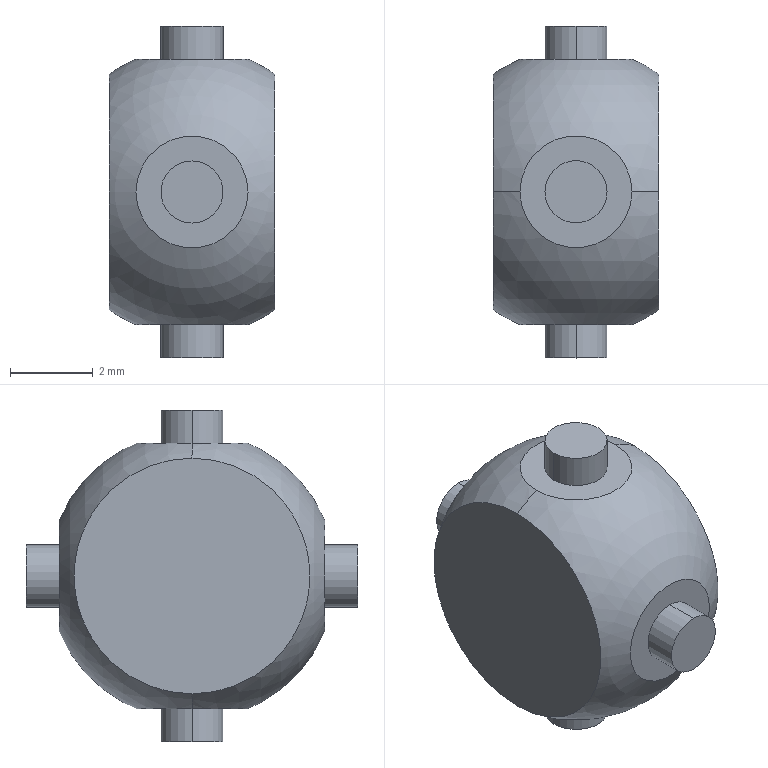Part | SolidWorks | features BaseBody 1, Scale 1 | 1 solid | 20 faces | box 4 x 8 x 8 mm | volume 137.312 mm3 | plane 10 | cylinder 8 | sphere 2 | commonest cylinder face diameters 1.5 x8
STEP:
#1=CARTESIAN_POINT('',(1.35,3.2,0.));
#2=VERTEX_POINT('',#1);
#3=CARTESIAN_POINT('',(-1.35,3.2,0.));
#4=VERTEX_POINT('',#3);
#5=CARTESIAN_POINT('',(0.,3.2,0.));
#6=DIRECTION('',(0.,1.,0.));
#7=DIRECTION('',(1.,0.,0.));
#8=AXIS2_PLACEMENT_3D('',#5,#6,#7);
#9=CIRCLE('',#8,1.35);
#10=EDGE_CURVE('',#2,#4,#9,.T.);
#11=ORIENTED_EDGE('',*,*,#10,.F.);
#12=CARTESIAN_POINT('',(0.,3.2,0.));
#13=DIRECTION('',(0.,1.,0.));
#14=DIRECTION('',(1.,0.,0.));
#15=AXIS2_PLACEMENT_3D('',#12,#13,#14);
#16=CIRCLE('',#15,1.35);
#17=EDGE_CURVE('',#4,#2,#16,.T.);
#18=ORIENTED_EDGE('',*,*,#17,.F.);
#19=EDGE_LOOP('',(#11,#18));
#20=FACE_BOUND('',#19,.T.);
#21=CARTESIAN_POINT('',(1.35,0.,-3.2));
#22=VERTEX_POINT('',#21);
#23=CARTESIAN_POINT('',(-1.35,0.,-3.2));
#24=VERTEX_POINT('',#23);
#25=CARTESIAN_POINT('',(0.,0.,-3.2));
#26=DIRECTION('',(0.,0.,1.));
#27=DIRECTION('',(1.,0.,0.));
#28=AXIS2_PLACEMENT_3D('',#25,#26,#27);
#29=CIRCLE('',#28,1.35);
#30=EDGE_CURVE('',#22,#24,#29,.T.);
#31=ORIENTED_EDGE('',*,*,#30,.T.);
#32=CARTESIAN_POINT('',(-2.,0.,-2.839));
#33=VERTEX_POINT('',#32);
#34=CARTESIAN_POINT('',(0.,0.,0.));
#35=DIRECTION('',(0.,1.,0.));
#36=DIRECTION('',(-1.,0.,0.));
#37=AXIS2_PLACEMENT_3D('',#34,#35,#36);
#38=CIRCLE('',#37,3.473);
#39=EDGE_CURVE('',#24,#33,#38,.T.);
#40=ORIENTED_EDGE('',*,*,#39,.T.);
#41=CARTESIAN_POINT('',(-2.,0.,2.839));
#42=VERTEX_POINT('',#41);
#43=CARTESIAN_POINT('',(-2.,0.,0.));
#44=DIRECTION('',(-1.,0.,0.));
#45=DIRECTION('',(0.,0.,-1.));
#46=AXIS2_PLACEMENT_3D('',#43,#44,#45);
#47=CIRCLE('',#46,2.839);
#48=EDGE_CURVE('',#42,#33,#47,.T.);
#49=ORIENTED_EDGE('',*,*,#48,.F.);
#50=CARTESIAN_POINT('',(-1.35,0.,3.2));
#51=VERTEX_POINT('',#50);
#52=CARTESIAN_POINT('',(0.,0.,0.));
#53=DIRECTION('',(0.,1.,0.));
#54=DIRECTION('',(-1.,0.,0.));
#55=AXIS2_PLACEMENT_3D('',#52,#53,#54);
#56=CIRCLE('',#55,3.473);
#57=EDGE_CURVE('',#42,#51,#56,.T.);
#58=ORIENTED_EDGE('',*,*,#57,.T.);
#59=CARTESIAN_POINT('',(1.35,0.,3.2));
#60=VERTEX_POINT('',#59);
#61=CARTESIAN_POINT('',(0.,0.,3.2));
#62=DIRECTION('',(0.,0.,1.));
#63=DIRECTION('',(1.,0.,0.));
#64=AXIS2_PLACEMENT_3D('',#61,#62,#63);
#65=CIRCLE('',#64,1.35);
#66=EDGE_CURVE('',#60,#51,#65,.T.);
#67=ORIENTED_EDGE('',*,*,#66,.F.);
#68=CARTESIAN_POINT('',(2.,0.,2.839));
#69=VERTEX_POINT('',#68);
#70=CARTESIAN_POINT('',(0.,0.,0.));
#71=DIRECTION('',(0.,-1.,0.));
#72=DIRECTION('',(0.,0.,-1.));
#73=AXIS2_PLACEMENT_3D('',#70,#71,#72);
#74=CIRCLE('',#73,3.473);
#75=EDGE_CURVE('',#69,#60,#74,.T.);
#76=ORIENTED_EDGE('',*,*,#75,.F.);
#77=CARTESIAN_POINT('',(2.,0.,-2.839));
#78=VERTEX_POINT('',#77);
#79=CARTESIAN_POINT('',(2.,0.,0.));
#80=DIRECTION('',(1.,0.,0.));
#81=DIRECTION('',(0.,0.,1.));
#82=AXIS2_PLACEMENT_3D('',#79,#80,#81);
#83=CIRCLE('',#82,2.839);
#84=EDGE_CURVE('',#78,#69,#83,.T.);
#85=ORIENTED_EDGE('',*,*,#84,.F.);
#86=CARTESIAN_POINT('',(0.,0.,0.));
#87=DIRECTION('',(0.,-1.,0.));
#88=DIRECTION('',(0.,0.,-1.));
#89=AXIS2_PLACEMENT_3D('',#86,#87,#88);
#90=CIRCLE('',#89,3.473);
#91=EDGE_CURVE('',#22,#78,#90,.T.);
#92=ORIENTED_EDGE('',*,*,#91,.F.);
#93=EDGE_LOOP('',(#31,#40,#49,#58,#67,#76,#85,#92));
#94=FACE_OUTER_BOUND('',#93,.T.);
#95=CARTESIAN_POINT('',(0.,0.,0.));
#96=DIRECTION('',(0.,1.,0.));
#97=DIRECTION('',(1.,0.,0.));
#98=AXIS2_PLACEMENT_3D('',#95,#96,#97);
#99=SPHERICAL_SURFACE('',#98,3.473);
#100=ADVANCED_FACE('',(#20,#94),#99,.T.);
#101=CARTESIAN_POINT('',(0.,3.2,-0.75));
#102=VERTEX_POINT('',#101);
#103=CARTESIAN_POINT('',(0.,3.2,0.75));
#104=VERTEX_POINT('',#103);
#105=CARTESIAN_POINT('',(0.,3.2,0.));
#106=DIRECTION('',(0.,-1.,0.));
#107=DIRECTION('',(1.,0.,0.));
#108=AXIS2_PLACEMENT_3D('',#105,#106,#107);
#109=CIRCLE('',#108,0.75);
#110=EDGE_CURVE('',#102,#104,#109,.T.);
#111=ORIENTED_EDGE('',*,*,#110,.F.);
#112=CARTESIAN_POINT('',(0.,4.,-0.75));
#113=VERTEX_POINT('',#112);
#114=CARTESIAN_POINT('',(0.,-4.,-0.75));
#115=DIRECTION('',(0.,1.,0.));
#116=VECTOR('',#115,1000.);
#117=LINE('',#114,#116);
#118=EDGE_CURVE('',#102,#113,#117,.T.);
#119=ORIENTED_EDGE('',*,*,#118,.T.);
#120=CARTESIAN_POINT('',(0.,4.,0.75));
#121=VERTEX_POINT('',#120);
#122=CARTESIAN_POINT('',(0.,4.,0.));
#123=DIRECTION('',(0.,1.,0.));
#124=DIRECTION('',(1.,0.,0.));
#125=AXIS2_PLACEMENT_3D('',#122,#123,#124);
#126=CIRCLE('',#125,0.75);
#127=EDGE_CURVE('',#121,#113,#126,.T.);
#128=ORIENTED_EDGE('',*,*,#127,.F.);
#129=CARTESIAN_POINT('',(0.,-4.,0.75));
#130=DIRECTION('',(0.,1.,0.));
#131=VECTOR('',#130,1000.);
#132=LINE('',#129,#131);
#133=EDGE_CURVE('',#104,#121,#132,.T.);
#134=ORIENTED_EDGE('',*,*,#133,.F.);
#135=EDGE_LOOP('',(#111,#119,#128,#134));
#136=FACE_OUTER_BOUND('',#135,.T.);
#137=CARTESIAN_POINT('',(0.,-4.,0.));
#138=DIRECTION('',(0.,1.,0.));
#139=DIRECTION('',(0.,0.,1.));
#140=AXIS2_PLACEMENT_3D('',#137,#138,#139);
#141=CYLINDRICAL_SURFACE('',#140,0.75);
#142=ADVANCED_FACE('',(#136),#141,.T.);
#143=CARTESIAN_POINT('',(0.,-4.,0.75));
#144=VERTEX_POINT('',#143);
#145=CARTESIAN_POINT('',(0.,-4.,-0.75));
#146=VERTEX_POINT('',#145);
#147=CARTESIAN_POINT('',(0.,-4.,0.));
#148=DIRECTION('',(0.,1.,0.));
#149=DIRECTION('',(1.,0.,0.));
#150=AXIS2_PLACEMENT_3D('',#147,#148,#149);
#151=CIRCLE('',#150,0.75);
#152=EDGE_CURVE('',#144,#146,#151,.T.);
#153=ORIENTED_EDGE('',*,*,#152,.T.);
#154=CARTESIAN_POINT('',(0.,-3.2,-0.75));
#155=VERTEX_POINT('',#154);
#156=CARTESIAN_POINT('',(0.,-4.,-0.75));
#157=DIRECTION('',(0.,1.,0.));
#158=VECTOR('',#157,1000.);
#159=LINE('',#156,#158);
#160=EDGE_CURVE('',#146,#155,#159,.T.);
#161=ORIENTED_EDGE('',*,*,#160,.T.);
#162=CARTESIAN_POINT('',(0.,-3.2,0.75));
#163=VERTEX_POINT('',#162);
#164=CARTESIAN_POINT('',(0.,-3.2,0.));
#165=DIRECTION('',(0.,1.,0.));
#166=DIRECTION('',(-1.,0.,0.));
#167=AXIS2_PLACEMENT_3D('',#164,#165,#166);
#168=CIRCLE('',#167,0.75);
#169=EDGE_CURVE('',#163,#155,#168,.T.);
#170=ORIENTED_EDGE('',*,*,#169,.F.);
#171=CARTESIAN_POINT('',(0.,-4.,0.75));
#172=DIRECTION('',(0.,1.,0.));
#173=VECTOR('',#172,1000.);
#174=LINE('',#171,#173);
#175=EDGE_CURVE('',#144,#163,#174,.T.);
#176=ORIENTED_EDGE('',*,*,#175,.F.);
#177=EDGE_LOOP('',(#153,#161,#170,#176));
#178=FACE_OUTER_BOUND('',#177,.T.);
#179=CARTESIAN_POINT('',(0.,-4.,0.));
#180=DIRECTION('',(0.,1.,0.));
#181=DIRECTION('',(0.,0.,1.));
#182=AXIS2_PLACEMENT_3D('',#179,#180,#181);
#183=CYLINDRICAL_SURFACE('',#182,0.75);
#184=ADVANCED_FACE('',(#178),#183,.T.);
#185=CARTESIAN_POINT('',(-0.75,0.,-3.2));
#186=VERTEX_POINT('',#185);
#187=CARTESIAN_POINT('',(0.75,0.,-3.2));
#188=VERTEX_POINT('',#187);
#189=CARTESIAN_POINT('',(0.,0.,-3.2));
#190=DIRECTION('',(0.,0.,-1.));
#191=DIRECTION('',(-1.,0.,0.));
#192=AXIS2_PLACEMENT_3D('',#189,#190,#191);
#193=CIRCLE('',#192,0.75);
#194=EDGE_CURVE('',#186,#188,#193,.T.);
#195=ORIENTED_EDGE('',*,*,#194,.T.);
#196=CARTESIAN_POINT('',(0.75,0.,-4.));
#197=VERTEX_POINT('',#196);
#198=CARTESIAN_POINT('',(0.75,0.,4.));
#199=DIRECTION('',(0.,0.,-1.));
#200=VECTOR('',#199,1000.);
#201=LINE('',#198,#200);
#202=EDGE_CURVE('',#188,#197,#201,.T.);
#203=ORIENTED_EDGE('',*,*,#202,.T.);
#204=CARTESIAN_POINT('',(-0.75,0.,-4.));
#205=VERTEX_POINT('',#204);
#206=CARTESIAN_POINT('',(0.,0.,-4.));
#207=DIRECTION('',(0.,0.,-1.));
#208=DIRECTION('',(1.,0.,0.));
#209=AXIS2_PLACEMENT_3D('',#206,#207,#208);
#210=CIRCLE('',#209,0.75);
#211=EDGE_CURVE('',#205,#197,#210,.T.);
#212=ORIENTED_EDGE('',*,*,#211,.F.);
#213=CARTESIAN_POINT('',(-0.75,0.,4.));
#214=DIRECTION('',(0.,0.,-1.));
#215=VECTOR('',#214,1000.);
#216=LINE('',#213,#215);
#217=EDGE_CURVE('',#186,#205,#216,.T.);
#218=ORIENTED_EDGE('',*,*,#217,.F.);
#219=EDGE_LOOP('',(#195,#203,#212,#218));
#220=FACE_OUTER_BOUND('',#219,.T.);
#221=CARTESIAN_POINT('',(0.,0.,4.));
#222=DIRECTION('',(0.,0.,-1.));
#223=DIRECTION('',(-1.,0.,0.));
#224=AXIS2_PLACEMENT_3D('',#221,#222,#223);
#225=CYLINDRICAL_SURFACE('',#224,0.75);
#226=ADVANCED_FACE('',(#220),#225,.T.);
#227=CARTESIAN_POINT('',(-0.75,0.,4.));
#228=VERTEX_POINT('',#227);
#229=CARTESIAN_POINT('',(0.75,0.,4.));
#230=VERTEX_POINT('',#229);
#231=CARTESIAN_POINT('',(0.,0.,4.));
#232=DIRECTION('',(0.,0.,-1.));
#233=DIRECTION('',(1.,0.,0.));
#234=AXIS2_PLACEMENT_3D('',#231,#232,#233);
#235=CIRCLE('',#234,0.75);
#236=EDGE_CURVE('',#228,#230,#235,.T.);
#237=ORIENTED_EDGE('',*,*,#236,.T.);
#238=CARTESIAN_POINT('',(0.75,0.,3.2));
#239=VERTEX_POINT('',#238);
#240=CARTESIAN_POINT('',(0.75,0.,4.));
#241=DIRECTION('',(0.,0.,-1.));
#242=VECTOR('',#241,1000.);
#243=LINE('',#240,#242);
#244=EDGE_CURVE('',#230,#239,#243,.T.);
#245=ORIENTED_EDGE('',*,*,#244,.T.);
#246=CARTESIAN_POINT('',(-0.75,0.,3.2));
#247=VERTEX_POINT('',#246);
#248=CARTESIAN_POINT('',(0.,0.,3.2));
#249=DIRECTION('',(0.,0.,1.));
#250=DIRECTION('',(1.,0.,0.));
#251=AXIS2_PLACEMENT_3D('',#248,#249,#250);
#252=CIRCLE('',#251,0.75);
#253=EDGE_CURVE('',#239,#247,#252,.T.);
#254=ORIENTED_EDGE('',*,*,#253,.T.);
#255=CARTESIAN_POINT('',(-0.75,0.,4.));
#256=DIRECTION('',(0.,0.,-1.));
#257=VECTOR('',#256,1000.);
#258=LINE('',#255,#257);
#259=EDGE_CURVE('',#228,#247,#258,.T.);
#260=ORIENTED_EDGE('',*,*,#259,.F.);
#261=EDGE_LOOP('',(#237,#245,#254,#260));
#262=FACE_OUTER_BOUND('',#261,.T.);
#263=CARTESIAN_POINT('',(0.,0.,4.));
#264=DIRECTION('',(0.,0.,-1.));
#265=DIRECTION('',(-1.,0.,0.));
#266=AXIS2_PLACEMENT_3D('',#263,#264,#265);
#267=CYLINDRICAL_SURFACE('',#266,0.75);
#268=ADVANCED_FACE('',(#262),#267,.T.);
#269=ORIENTED_EDGE('',*,*,#236,.F.);
#270=CARTESIAN_POINT('',(0.,0.,4.));
#271=DIRECTION('',(0.,0.,-1.));
#272=DIRECTION('',(1.,0.,0.));
#273=AXIS2_PLACEMENT_3D('',#270,#271,#272);
#274=CIRCLE('',#273,0.75);
#275=EDGE_CURVE('',#230,#228,#274,.T.);
#276=ORIENTED_EDGE('',*,*,#275,.F.);
#277=EDGE_LOOP('',(#269,#276));
#278=FACE_OUTER_BOUND('',#277,.T.);
#279=CARTESIAN_POINT('',(0.,0.,4.));
#280=DIRECTION('',(0.,0.,-1.));
#281=DIRECTION('',(0.,-1.,0.));
#282=AXIS2_PLACEMENT_3D('',#279,#280,#281);
#283=PLANE('',#282);
#284=ADVANCED_FACE('',(#278),#283,.F.);
#285=ORIENTED_EDGE('',*,*,#244,.F.);
#286=ORIENTED_EDGE('',*,*,#275,.T.);
#287=ORIENTED_EDGE('',*,*,#259,.T.);
#288=CARTESIAN_POINT('',(0.,0.,3.2));
#289=DIRECTION('',(0.,0.,1.));
#290=DIRECTION('',(1.,0.,0.));
#291=AXIS2_PLACEMENT_3D('',#288,#289,#290);
#292=CIRCLE('',#291,0.75);
#293=EDGE_CURVE('',#247,#239,#292,.T.);
#294=ORIENTED_EDGE('',*,*,#293,.T.);
#295=EDGE_LOOP('',(#285,#286,#287,#294));
#296=FACE_OUTER_BOUND('',#295,.T.);
#297=CARTESIAN_POINT('',(0.,0.,4.));
#298=DIRECTION('',(0.,0.,-1.));
#299=DIRECTION('',(-1.,0.,0.));
#300=AXIS2_PLACEMENT_3D('',#297,#298,#299);
#301=CYLINDRICAL_SURFACE('',#300,0.75);
#302=ADVANCED_FACE('',(#296),#301,.T.);
#303=ORIENTED_EDGE('',*,*,#202,.F.);
#304=CARTESIAN_POINT('',(0.,0.,-3.2));
#305=DIRECTION('',(0.,0.,-1.));
#306=DIRECTION('',(-1.,0.,0.));
#307=AXIS2_PLACEMENT_3D('',#304,#305,#306);
#308=CIRCLE('',#307,0.75);
#309=EDGE_CURVE('',#188,#186,#308,.T.);
#310=ORIENTED_EDGE('',*,*,#309,.T.);
#311=ORIENTED_EDGE('',*,*,#217,.T.);
#312=CARTESIAN_POINT('',(0.,0.,-4.));
#313=DIRECTION('',(0.,0.,-1.));
#314=DIRECTION('',(1.,0.,0.));
#315=AXIS2_PLACEMENT_3D('',#312,#313,#314);
#316=CIRCLE('',#315,0.75);
#317=EDGE_CURVE('',#197,#205,#316,.T.);
#318=ORIENTED_EDGE('',*,*,#317,.F.);
#319=EDGE_LOOP('',(#303,#310,#311,#318));
#320=FACE_OUTER_BOUND('',#319,.T.);
#321=CARTESIAN_POINT('',(0.,0.,4.));
#322=DIRECTION('',(0.,0.,-1.));
#323=DIRECTION('',(-1.,0.,0.));
#324=AXIS2_PLACEMENT_3D('',#321,#322,#323);
#325=CYLINDRICAL_SURFACE('',#324,0.75);
#326=ADVANCED_FACE('',(#320),#325,.T.);
#327=ORIENTED_EDGE('',*,*,#211,.T.);
#328=ORIENTED_EDGE('',*,*,#317,.T.);
#329=EDGE_LOOP('',(#327,#328));
#330=FACE_OUTER_BOUND('',#329,.T.);
#331=CARTESIAN_POINT('',(0.,0.,-4.));
#332=DIRECTION('',(0.,0.,-1.));
#333=DIRECTION('',(0.,-1.,0.));
#334=AXIS2_PLACEMENT_3D('',#331,#332,#333);
#335=PLANE('',#334);
#336=ADVANCED_FACE('',(#330),#335,.T.);
#337=ORIENTED_EDGE('',*,*,#152,.F.);
#338=CARTESIAN_POINT('',(0.,-4.,0.));
#339=DIRECTION('',(0.,1.,0.));
#340=DIRECTION('',(1.,0.,0.));
#341=AXIS2_PLACEMENT_3D('',#338,#339,#340);
#342=CIRCLE('',#341,0.75);
#343=EDGE_CURVE('',#146,#144,#342,.T.);
#344=ORIENTED_EDGE('',*,*,#343,.F.);
#345=EDGE_LOOP('',(#337,#344));
#346=FACE_OUTER_BOUND('',#345,.T.);
#347=CARTESIAN_POINT('',(0.,-4.,0.));
#348=DIRECTION('',(0.,1.,0.));
#349=DIRECTION('',(1.,0.,0.));
#350=AXIS2_PLACEMENT_3D('',#347,#348,#349);
#351=PLANE('',#350);
#352=ADVANCED_FACE('',(#346),#351,.F.);
#353=ORIENTED_EDGE('',*,*,#160,.F.);
#354=ORIENTED_EDGE('',*,*,#343,.T.);
#355=ORIENTED_EDGE('',*,*,#175,.T.);
#356=CARTESIAN_POINT('',(0.,-3.2,0.));
#357=DIRECTION('',(0.,1.,0.));
#358=DIRECTION('',(-1.,0.,0.));
#359=AXIS2_PLACEMENT_3D('',#356,#357,#358);
#360=CIRCLE('',#359,0.75);
#361=EDGE_CURVE('',#155,#163,#360,.T.);
#362=ORIENTED_EDGE('',*,*,#361,.F.);
#363=EDGE_LOOP('',(#353,#354,#355,#362));
#364=FACE_OUTER_BOUND('',#363,.T.);
#365=CARTESIAN_POINT('',(0.,-4.,0.));
#366=DIRECTION('',(0.,1.,0.));
#367=DIRECTION('',(0.,0.,1.));
#368=AXIS2_PLACEMENT_3D('',#365,#366,#367);
#369=CYLINDRICAL_SURFACE('',#368,0.75);
#370=ADVANCED_FACE('',(#364),#369,.T.);
#371=ORIENTED_EDGE('',*,*,#118,.F.);
#372=CARTESIAN_POINT('',(0.,3.2,0.));
#373=DIRECTION('',(0.,-1.,0.));
#374=DIRECTION('',(1.,0.,0.));
#375=AXIS2_PLACEMENT_3D('',#372,#373,#374);
#376=CIRCLE('',#375,0.75);
#377=EDGE_CURVE('',#104,#102,#376,.T.);
#378=ORIENTED_EDGE('',*,*,#377,.F.);
#379=ORIENTED_EDGE('',*,*,#133,.T.);
#380=CARTESIAN_POINT('',(0.,4.,0.));
#381=DIRECTION('',(0.,1.,0.));
#382=DIRECTION('',(1.,0.,0.));
#383=AXIS2_PLACEMENT_3D('',#380,#381,#382);
#384=CIRCLE('',#383,0.75);
#385=EDGE_CURVE('',#113,#121,#384,.T.);
#386=ORIENTED_EDGE('',*,*,#385,.F.);
#387=EDGE_LOOP('',(#371,#378,#379,#386));
#388=FACE_OUTER_BOUND('',#387,.T.);
#389=CARTESIAN_POINT('',(0.,-4.,0.));
#390=DIRECTION('',(0.,1.,0.));
#391=DIRECTION('',(0.,0.,1.));
#392=AXIS2_PLACEMENT_3D('',#389,#390,#391);
#393=CYLINDRICAL_SURFACE('',#392,0.75);
#394=ADVANCED_FACE('',(#388),#393,.T.);
#395=ORIENTED_EDGE('',*,*,#127,.T.);
#396=ORIENTED_EDGE('',*,*,#385,.T.);
#397=EDGE_LOOP('',(#395,#396));
#398=FACE_OUTER_BOUND('',#397,.T.);
#399=CARTESIAN_POINT('',(0.,4.,0.));
#400=DIRECTION('',(0.,1.,0.));
#401=DIRECTION('',(1.,0.,0.));
#402=AXIS2_PLACEMENT_3D('',#399,#400,#401);
#403=PLANE('',#402);
#404=ADVANCED_FACE('',(#398),#403,.T.);
#405=ORIENTED_EDGE('',*,*,#10,.T.);
#406=ORIENTED_EDGE('',*,*,#17,.T.);
#407=EDGE_LOOP('',(#405,#406));
#408=FACE_OUTER_BOUND('',#407,.T.);
#409=ORIENTED_EDGE('',*,*,#377,.T.);
#410=ORIENTED_EDGE('',*,*,#110,.T.);
#411=EDGE_LOOP('',(#409,#410));
#412=FACE_BOUND('',#411,.T.);
#413=CARTESIAN_POINT('',(2.,3.2,3.2));
#414=DIRECTION('',(0.,-1.,0.));
#415=DIRECTION('',(-1.,0.,0.));
#416=AXIS2_PLACEMENT_3D('',#413,#414,#415);
#417=PLANE('',#416);
#418=ADVANCED_FACE('',(#408,#412),#417,.F.);
#419=CARTESIAN_POINT('',(2.,0.,0.));
#420=DIRECTION('',(1.,0.,0.));
#421=DIRECTION('',(0.,0.,1.));
#422=AXIS2_PLACEMENT_3D('',#419,#420,#421);
#423=CIRCLE('',#422,2.839);
#424=EDGE_CURVE('',#69,#78,#423,.T.);
#425=ORIENTED_EDGE('',*,*,#424,.T.);
#426=ORIENTED_EDGE('',*,*,#84,.T.);
#427=EDGE_LOOP('',(#425,#426));
#428=FACE_OUTER_BOUND('',#427,.T.);
#429=CARTESIAN_POINT('',(2.,-3.2,3.2));
#430=DIRECTION('',(-1.,0.,0.));
#431=DIRECTION('',(0.,0.,1.));
#432=AXIS2_PLACEMENT_3D('',#429,#430,#431);
#433=PLANE('',#432);
#434=ADVANCED_FACE('',(#428),#433,.F.);
#435=CARTESIAN_POINT('',(-1.35,-3.2,0.));
#436=VERTEX_POINT('',#435);
#437=CARTESIAN_POINT('',(1.35,-3.2,0.));
#438=VERTEX_POINT('',#437);
#439=CARTESIAN_POINT('',(0.,-3.2,0.));
#440=DIRECTION('',(0.,-1.,0.));
#441=DIRECTION('',(-1.,0.,0.));
#442=AXIS2_PLACEMENT_3D('',#439,#440,#441);
#443=CIRCLE('',#442,1.35);
#444=EDGE_CURVE('',#436,#438,#443,.T.);
#445=ORIENTED_EDGE('',*,*,#444,.T.);
#446=CARTESIAN_POINT('',(0.,-3.2,0.));
#447=DIRECTION('',(0.,-1.,0.));
#448=DIRECTION('',(-1.,0.,0.));
#449=AXIS2_PLACEMENT_3D('',#446,#447,#448);
#450=CIRCLE('',#449,1.35);
#451=EDGE_CURVE('',#438,#436,#450,.T.);
#452=ORIENTED_EDGE('',*,*,#451,.T.);
#453=EDGE_LOOP('',(#445,#452));
#454=FACE_OUTER_BOUND('',#453,.T.);
#455=ORIENTED_EDGE('',*,*,#169,.T.);
#456=ORIENTED_EDGE('',*,*,#361,.T.);
#457=EDGE_LOOP('',(#455,#456));
#458=FACE_BOUND('',#457,.T.);
#459=CARTESIAN_POINT('',(-2.,-3.2,3.2));
#460=DIRECTION('',(0.,1.,0.));
#461=DIRECTION('',(1.,0.,0.));
#462=AXIS2_PLACEMENT_3D('',#459,#460,#461);
#463=PLANE('',#462);
#464=ADVANCED_FACE('',(#454,#458),#463,.F.);
#465=CARTESIAN_POINT('',(-2.,0.,0.));
#466=DIRECTION('',(-1.,0.,0.));
#467=DIRECTION('',(0.,0.,-1.));
#468=AXIS2_PLACEMENT_3D('',#465,#466,#467);
#469=CIRCLE('',#468,2.839);
#470=EDGE_CURVE('',#33,#42,#469,.T.);
#471=ORIENTED_EDGE('',*,*,#470,.T.);
#472=ORIENTED_EDGE('',*,*,#48,.T.);
#473=EDGE_LOOP('',(#471,#472));
#474=FACE_OUTER_BOUND('',#473,.T.);
#475=CARTESIAN_POINT('',(-2.,3.2,3.2));
#476=DIRECTION('',(1.,0.,0.));
#477=DIRECTION('',(0.,1.,0.));
#478=AXIS2_PLACEMENT_3D('',#475,#476,#477);
#479=PLANE('',#478);
#480=ADVANCED_FACE('',(#474),#479,.F.);
#481=ORIENTED_EDGE('',*,*,#30,.F.);
#482=CARTESIAN_POINT('',(0.,0.,-3.2));
#483=DIRECTION('',(0.,0.,1.));
#484=DIRECTION('',(1.,0.,0.));
#485=AXIS2_PLACEMENT_3D('',#482,#483,#484);
#486=CIRCLE('',#485,1.35);
#487=EDGE_CURVE('',#24,#22,#486,.T.);
#488=ORIENTED_EDGE('',*,*,#487,.F.);
#489=EDGE_LOOP('',(#481,#488));
#490=FACE_OUTER_BOUND('',#489,.T.);
#491=ORIENTED_EDGE('',*,*,#194,.F.);
#492=ORIENTED_EDGE('',*,*,#309,.F.);
#493=EDGE_LOOP('',(#491,#492));
#494=FACE_BOUND('',#493,.T.);
#495=CARTESIAN_POINT('',(0.,0.,-3.2));
#496=DIRECTION('',(0.,0.,-1.));
#497=DIRECTION('',(0.,-1.,0.));
#498=AXIS2_PLACEMENT_3D('',#495,#496,#497);
#499=PLANE('',#498);
#500=ADVANCED_FACE('',(#490,#494),#499,.T.);
#501=ORIENTED_EDGE('',*,*,#39,.F.);
#502=ORIENTED_EDGE('',*,*,#487,.T.);
#503=ORIENTED_EDGE('',*,*,#91,.T.);
#504=ORIENTED_EDGE('',*,*,#424,.F.);
#505=ORIENTED_EDGE('',*,*,#75,.T.);
#506=CARTESIAN_POINT('',(0.,0.,3.2));
#507=DIRECTION('',(0.,0.,1.));
#508=DIRECTION('',(1.,0.,0.));
#509=AXIS2_PLACEMENT_3D('',#506,#507,#508);
#510=CIRCLE('',#509,1.35);
#511=EDGE_CURVE('',#51,#60,#510,.T.);
#512=ORIENTED_EDGE('',*,*,#511,.F.);
#513=ORIENTED_EDGE('',*,*,#57,.F.);
#514=ORIENTED_EDGE('',*,*,#470,.F.);
#515=EDGE_LOOP('',(#501,#502,#503,#504,#505,#512,#513,#514));
#516=FACE_OUTER_BOUND('',#515,.T.);
#517=ORIENTED_EDGE('',*,*,#444,.F.);
#518=ORIENTED_EDGE('',*,*,#451,.F.);
#519=EDGE_LOOP('',(#517,#518));
#520=FACE_BOUND('',#519,.T.);
#521=CARTESIAN_POINT('',(0.,0.,0.));
#522=DIRECTION('',(0.,1.,0.));
#523=DIRECTION('',(1.,0.,0.));
#524=AXIS2_PLACEMENT_3D('',#521,#522,#523);
#525=SPHERICAL_SURFACE('',#524,3.473);
#526=ADVANCED_FACE('',(#516,#520),#525,.T.);
#527=ORIENTED_EDGE('',*,*,#66,.T.);
#528=ORIENTED_EDGE('',*,*,#511,.T.);
#529=EDGE_LOOP('',(#527,#528));
#530=FACE_OUTER_BOUND('',#529,.T.);
#531=ORIENTED_EDGE('',*,*,#293,.F.);
#532=ORIENTED_EDGE('',*,*,#253,.F.);
#533=EDGE_LOOP('',(#531,#532));
#534=FACE_BOUND('',#533,.T.);
#535=CARTESIAN_POINT('',(0.,0.,3.2));
#536=DIRECTION('',(0.,0.,1.));
#537=DIRECTION('',(1.,0.,0.));
#538=AXIS2_PLACEMENT_3D('',#535,#536,#537);
#539=PLANE('',#538);
#540=ADVANCED_FACE('',(#530,#534),#539,.T.);
#541=CLOSED_SHELL('',(#100,#142,#184,#226,#268,#284,#302,#326,#336,#352,#370,#394,#404,#418,#434,#464,#480,#500,#526,#540));
#542=MANIFOLD_SOLID_BREP('',#541);
#543=CARTESIAN_POINT('',(0.,0.,0.));
#544=DIRECTION('',(0.,0.,1.));
#545=DIRECTION('',(1.,0.,0.));
#546=AXIS2_PLACEMENT_3D('',#543,#544,#545);
#547=(LENGTH_UNIT()NAMED_UNIT(*)SI_UNIT(.MILLI.,.METRE.));
#548=UNCERTAINTY_MEASURE_WITH_UNIT(LENGTH_MEASURE(0.00001),#547,'','');
#549=(NAMED_UNIT(*)PLANE_ANGLE_UNIT()SI_UNIT($,.RADIAN.));
#550=(NAMED_UNIT(*)SI_UNIT($,.STERADIAN.)SOLID_ANGLE_UNIT());
#551=(GEOMETRIC_REPRESENTATION_CONTEXT(3)GLOBAL_UNCERTAINTY_ASSIGNED_CONTEXT((#548))GLOBAL_UNIT_ASSIGNED_CONTEXT((#547,#549,#550))REPRESENTATION_CONTEXT('',''));
#552=ADVANCED_BREP_SHAPE_REPRESENTATION('',(#542,#546),#551);